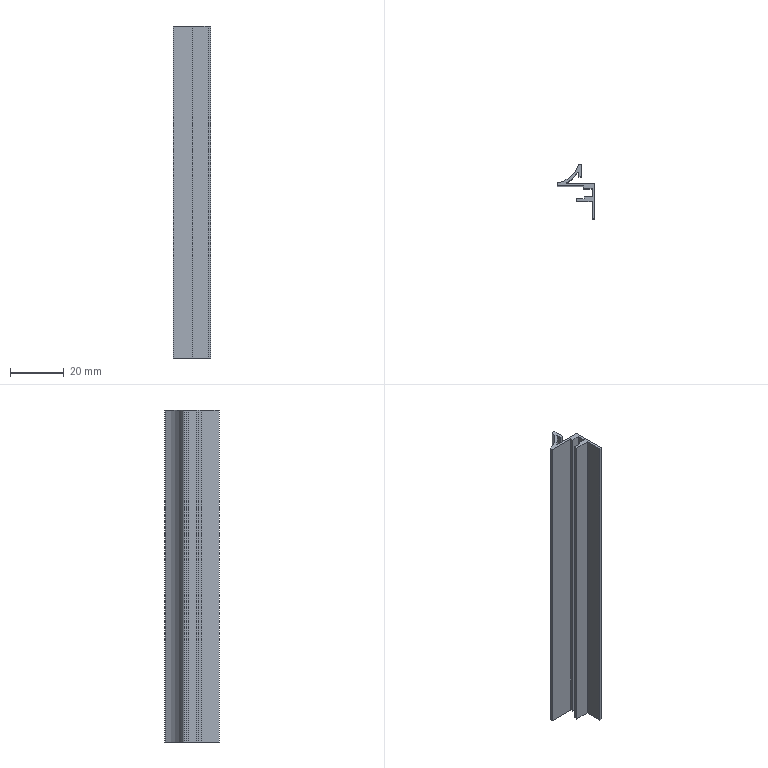Part | SolidWorks | features BaseBody 1, ICE 1, MoveFace 1 | 1 solid | 27 faces | box 14 x 20.3 x 124 mm | volume 6314 mm3 | plane 20 | cylinder 7 | commonest cylinder face diameters 0.387 x2 0.8 x2 0.4 x1 20 x1 22 x1
STEP:
#1=CARTESIAN_POINT('',(-5.304,-0.625,200.));
#2=VERTEX_POINT('',#1);
#3=CARTESIAN_POINT('',(-5.449,-0.8125,200.));
#4=VERTEX_POINT('',#3);
#5=CARTESIAN_POINT('',(-5.255,-0.8125,200.));
#6=DIRECTION('',(0.,0.,1.));
#7=DIRECTION('',(-1.,0.,0.));
#8=AXIS2_PLACEMENT_3D('',#5,#6,#7);
#9=CIRCLE('',#8,0.1937);
#10=EDGE_CURVE('',#2,#4,#9,.T.);
#11=ORIENTED_EDGE('',*,*,#10,.T.);
#12=CARTESIAN_POINT('',(-5.449,-0.8125,76.));
#13=VERTEX_POINT('',#12);
#14=CARTESIAN_POINT('',(-5.449,-0.8125,230.));
#15=DIRECTION('',(0.,0.,-1.));
#16=VECTOR('',#15,1000.);
#17=LINE('',#14,#16);
#18=EDGE_CURVE('',#4,#13,#17,.T.);
#19=ORIENTED_EDGE('',*,*,#18,.T.);
#20=CARTESIAN_POINT('',(-5.304,-0.625,76.));
#21=VERTEX_POINT('',#20);
#22=CARTESIAN_POINT('',(-5.255,-0.8125,76.));
#23=DIRECTION('',(0.,0.,-1.));
#24=DIRECTION('',(1.,0.,0.));
#25=AXIS2_PLACEMENT_3D('',#22,#23,#24);
#26=CIRCLE('',#25,0.1937);
#27=EDGE_CURVE('',#13,#21,#26,.T.);
#28=ORIENTED_EDGE('',*,*,#27,.T.);
#29=CARTESIAN_POINT('',(-5.304,-0.625,230.));
#30=DIRECTION('',(0.,0.,-1.));
#31=VECTOR('',#30,1000.);
#32=LINE('',#29,#31);
#33=EDGE_CURVE('',#2,#21,#32,.T.);
#34=ORIENTED_EDGE('',*,*,#33,.F.);
#35=EDGE_LOOP('',(#11,#19,#28,#34));
#36=FACE_OUTER_BOUND('',#35,.T.);
#37=CARTESIAN_POINT('',(-5.255,-0.8125,230.));
#38=DIRECTION('',(0.,0.,-1.));
#39=DIRECTION('',(-1.,0.,0.));
#40=AXIS2_PLACEMENT_3D('',#37,#38,#39);
#41=CYLINDRICAL_SURFACE('',#40,0.1937);
#42=ADVANCED_FACE('',(#36),#41,.F.);
#43=CARTESIAN_POINT('',(5.,-1.,76.));
#44=VERTEX_POINT('',#43);
#45=CARTESIAN_POINT('',(5.,-14.3,76.));
#46=VERTEX_POINT('',#45);
#47=CARTESIAN_POINT('',(5.,29.623,76.));
#48=DIRECTION('',(0.,-1.,0.));
#49=VECTOR('',#48,1000.);
#50=LINE('',#47,#49);
#51=EDGE_CURVE('',#44,#46,#50,.T.);
#52=ORIENTED_EDGE('',*,*,#51,.F.);
#53=CARTESIAN_POINT('',(5.,-1.,200.));
#54=VERTEX_POINT('',#53);
#55=CARTESIAN_POINT('',(5.,-1.,230.));
#56=DIRECTION('',(0.,0.,-1.));
#57=VECTOR('',#56,1000.);
#58=LINE('',#55,#57);
#59=EDGE_CURVE('',#54,#44,#58,.T.);
#60=ORIENTED_EDGE('',*,*,#59,.F.);
#61=CARTESIAN_POINT('',(5.,-14.3,200.));
#62=VERTEX_POINT('',#61);
#63=CARTESIAN_POINT('',(5.,-14.3,200.));
#64=DIRECTION('',(0.,1.,0.));
#65=VECTOR('',#64,1000.);
#66=LINE('',#63,#65);
#67=EDGE_CURVE('',#62,#54,#66,.T.);
#68=ORIENTED_EDGE('',*,*,#67,.F.);
#69=CARTESIAN_POINT('',(5.,-14.3,230.));
#70=DIRECTION('',(0.,0.,1.));
#71=VECTOR('',#70,1000.);
#72=LINE('',#69,#71);
#73=EDGE_CURVE('',#46,#62,#72,.T.);
#74=ORIENTED_EDGE('',*,*,#73,.F.);
#75=EDGE_LOOP('',(#52,#60,#68,#74));
#76=FACE_OUTER_BOUND('',#75,.T.);
#77=CARTESIAN_POINT('',(5.,-14.3,230.));
#78=DIRECTION('',(-1.,0.,0.));
#79=DIRECTION('',(0.,0.,1.));
#80=AXIS2_PLACEMENT_3D('',#77,#78,#79);
#81=PLANE('',#80);
#82=ADVANCED_FACE('',(#76),#81,.F.);
#83=CARTESIAN_POINT('',(-9.,-2.,76.));
#84=VERTEX_POINT('',#83);
#85=CARTESIAN_POINT('',(-9.,-2.,200.));
#86=VERTEX_POINT('',#85);
#87=CARTESIAN_POINT('',(-9.,-2.,230.));
#88=DIRECTION('',(0.,0.,1.));
#89=VECTOR('',#88,1000.);
#90=LINE('',#87,#89);
#91=EDGE_CURVE('',#84,#86,#90,.T.);
#92=ORIENTED_EDGE('',*,*,#91,.F.);
#93=CARTESIAN_POINT('',(0.9,-2.,76.));
#94=VERTEX_POINT('',#93);
#95=CARTESIAN_POINT('',(5.,-2.,76.));
#96=DIRECTION('',(-1.,0.,0.));
#97=VECTOR('',#96,1000.);
#98=LINE('',#95,#97);
#99=EDGE_CURVE('',#94,#84,#98,.T.);
#100=ORIENTED_EDGE('',*,*,#99,.F.);
#101=CARTESIAN_POINT('',(0.9,-2.,200.));
#102=VERTEX_POINT('',#101);
#103=CARTESIAN_POINT('',(0.9,-2.,230.));
#104=DIRECTION('',(0.,0.,-1.));
#105=VECTOR('',#104,1000.);
#106=LINE('',#103,#105);
#107=EDGE_CURVE('',#102,#94,#106,.T.);
#108=ORIENTED_EDGE('',*,*,#107,.F.);
#109=CARTESIAN_POINT('',(5.,-2.,200.));
#110=DIRECTION('',(1.,0.,0.));
#111=VECTOR('',#110,1000.);
#112=LINE('',#109,#111);
#113=EDGE_CURVE('',#86,#102,#112,.T.);
#114=ORIENTED_EDGE('',*,*,#113,.F.);
#115=EDGE_LOOP('',(#92,#100,#108,#114));
#116=FACE_OUTER_BOUND('',#115,.T.);
#117=CARTESIAN_POINT('',(-9.,-2.,230.));
#118=DIRECTION('',(0.,1.,0.));
#119=DIRECTION('',(0.,0.,1.));
#120=AXIS2_PLACEMENT_3D('',#117,#118,#119);
#121=PLANE('',#120);
#122=ADVANCED_FACE('',(#116),#121,.F.);
#123=CARTESIAN_POINT('',(4.,-6.,200.));
#124=VERTEX_POINT('',#123);
#125=CARTESIAN_POINT('',(4.,-3.,200.));
#126=VERTEX_POINT('',#125);
#127=CARTESIAN_POINT('',(4.,29.623,200.));
#128=DIRECTION('',(0.,1.,0.));
#129=VECTOR('',#128,1000.);
#130=LINE('',#127,#129);
#131=EDGE_CURVE('',#124,#126,#130,.T.);
#132=ORIENTED_EDGE('',*,*,#131,.F.);
#133=CARTESIAN_POINT('',(1.,-6.,200.));
#134=VERTEX_POINT('',#133);
#135=CARTESIAN_POINT('',(5.,-6.,200.));
#136=DIRECTION('',(1.,0.,0.));
#137=VECTOR('',#136,1000.);
#138=LINE('',#135,#137);
#139=EDGE_CURVE('',#134,#124,#138,.T.);
#140=ORIENTED_EDGE('',*,*,#139,.F.);
#141=CARTESIAN_POINT('',(1.,-6.7,200.));
#142=VERTEX_POINT('',#141);
#143=CARTESIAN_POINT('',(1.,-6.,200.));
#144=DIRECTION('',(0.,-1.,0.));
#145=VECTOR('',#144,1000.);
#146=LINE('',#143,#145);
#147=EDGE_CURVE('',#134,#142,#146,.T.);
#148=ORIENTED_EDGE('',*,*,#147,.T.);
#149=CARTESIAN_POINT('',(-1.7,-6.7,200.));
#150=VERTEX_POINT('',#149);
#151=CARTESIAN_POINT('',(5.,-6.7,200.));
#152=DIRECTION('',(1.,0.,0.));
#153=VECTOR('',#152,1000.);
#154=LINE('',#151,#153);
#155=EDGE_CURVE('',#150,#142,#154,.T.);
#156=ORIENTED_EDGE('',*,*,#155,.F.);
#157=CARTESIAN_POINT('',(-1.7,-7.7,200.));
#158=VERTEX_POINT('',#157);
#159=CARTESIAN_POINT('',(-1.7,-6.7,200.));
#160=DIRECTION('',(0.,-1.,0.));
#161=VECTOR('',#160,1000.);
#162=LINE('',#159,#161);
#163=EDGE_CURVE('',#150,#158,#162,.T.);
#164=ORIENTED_EDGE('',*,*,#163,.T.);
#165=CARTESIAN_POINT('',(4.,-7.7,200.));
#166=VERTEX_POINT('',#165);
#167=CARTESIAN_POINT('',(5.,-7.7,200.));
#168=DIRECTION('',(-1.,0.,0.));
#169=VECTOR('',#168,1000.);
#170=LINE('',#167,#169);
#171=EDGE_CURVE('',#166,#158,#170,.T.);
#172=ORIENTED_EDGE('',*,*,#171,.F.);
#173=CARTESIAN_POINT('',(4.,-14.3,200.));
#174=VERTEX_POINT('',#173);
#175=CARTESIAN_POINT('',(4.,29.623,200.));
#176=DIRECTION('',(0.,1.,0.));
#177=VECTOR('',#176,1000.);
#178=LINE('',#175,#177);
#179=EDGE_CURVE('',#174,#166,#178,.T.);
#180=ORIENTED_EDGE('',*,*,#179,.F.);
#181=CARTESIAN_POINT('',(5.,-14.3,200.));
#182=DIRECTION('',(-1.,0.,0.));
#183=VECTOR('',#182,1000.);
#184=LINE('',#181,#183);
#185=EDGE_CURVE('',#62,#174,#184,.T.);
#186=ORIENTED_EDGE('',*,*,#185,.F.);
#187=ORIENTED_EDGE('',*,*,#67,.T.);
#188=CARTESIAN_POINT('',(-5.207,-1.,200.));
#189=VERTEX_POINT('',#188);
#190=CARTESIAN_POINT('',(5.,-1.,200.));
#191=DIRECTION('',(1.,0.,0.));
#192=VECTOR('',#191,1000.);
#193=LINE('',#190,#192);
#194=EDGE_CURVE('',#189,#54,#193,.T.);
#195=ORIENTED_EDGE('',*,*,#194,.F.);
#196=CARTESIAN_POINT('',(-5.255,-0.8125,200.));
#197=DIRECTION('',(0.,0.,1.));
#198=DIRECTION('',(-1.,0.,0.));
#199=AXIS2_PLACEMENT_3D('',#196,#197,#198);
#200=CIRCLE('',#199,0.1937);
#201=EDGE_CURVE('',#4,#189,#200,.T.);
#202=ORIENTED_EDGE('',*,*,#201,.F.);
#203=ORIENTED_EDGE('',*,*,#10,.F.);
#204=CARTESIAN_POINT('',(-1.368,3.063,200.));
#205=VERTEX_POINT('',#204);
#206=CARTESIAN_POINT('',(-10.628,9.,200.));
#207=DIRECTION('',(0.,0.,1.));
#208=DIRECTION('',(-1.,0.,0.));
#209=AXIS2_PLACEMENT_3D('',#206,#207,#208);
#210=CIRCLE('',#209,11.);
#211=EDGE_CURVE('',#2,#205,#210,.T.);
#212=ORIENTED_EDGE('',*,*,#211,.T.);
#213=CARTESIAN_POINT('',(-1.,2.955,200.));
#214=VERTEX_POINT('',#213);
#215=CARTESIAN_POINT('',(-1.2,2.955,200.));
#216=DIRECTION('',(0.,0.,1.));
#217=DIRECTION('',(-1.,0.,0.));
#218=AXIS2_PLACEMENT_3D('',#215,#216,#217);
#219=CIRCLE('',#218,0.2);
#220=EDGE_CURVE('',#214,#205,#219,.T.);
#221=ORIENTED_EDGE('',*,*,#220,.F.);
#222=CARTESIAN_POINT('',(-1.,1.5,200.));
#223=VERTEX_POINT('',#222);
#224=CARTESIAN_POINT('',(-1.,2.955,200.));
#225=DIRECTION('',(0.,1.,0.));
#226=VECTOR('',#225,1000.);
#227=LINE('',#224,#226);
#228=EDGE_CURVE('',#223,#214,#227,.T.);
#229=ORIENTED_EDGE('',*,*,#228,.F.);
#230=CARTESIAN_POINT('',(0.,1.5,200.));
#231=VERTEX_POINT('',#230);
#232=CARTESIAN_POINT('',(-1.,1.5,200.));
#233=DIRECTION('',(-1.,0.,0.));
#234=VECTOR('',#233,1000.);
#235=LINE('',#232,#234);
#236=EDGE_CURVE('',#231,#223,#235,.T.);
#237=ORIENTED_EDGE('',*,*,#236,.F.);
#238=CARTESIAN_POINT('',(0.,6.,200.));
#239=VERTEX_POINT('',#238);
#240=CARTESIAN_POINT('',(0.,1.5,200.));
#241=DIRECTION('',(0.,-1.,0.));
#242=VECTOR('',#241,1000.);
#243=LINE('',#240,#242);
#244=EDGE_CURVE('',#239,#231,#243,.T.);
#245=ORIENTED_EDGE('',*,*,#244,.F.);
#246=CARTESIAN_POINT('',(-0.8,6.,200.));
#247=VERTEX_POINT('',#246);
#248=CARTESIAN_POINT('',(0.,6.,200.));
#249=DIRECTION('',(1.,0.,0.));
#250=VECTOR('',#249,1000.);
#251=LINE('',#248,#250);
#252=EDGE_CURVE('',#247,#239,#251,.T.);
#253=ORIENTED_EDGE('',*,*,#252,.F.);
#254=CARTESIAN_POINT('',(-1.178,5.731,200.));
#255=VERTEX_POINT('',#254);
#256=CARTESIAN_POINT('',(-0.8,5.6,200.));
#257=DIRECTION('',(0.,0.,1.));
#258=DIRECTION('',(-1.,0.,0.));
#259=AXIS2_PLACEMENT_3D('',#256,#257,#258);
#260=CIRCLE('',#259,0.4);
#261=EDGE_CURVE('',#247,#255,#260,.T.);
#262=ORIENTED_EDGE('',*,*,#261,.T.);
#263=CARTESIAN_POINT('',(-8.678,-0.8077,200.));
#264=VERTEX_POINT('',#263);
#265=CARTESIAN_POINT('',(-10.628,9.,200.));
#266=DIRECTION('',(0.,0.,1.));
#267=DIRECTION('',(-1.,0.,0.));
#268=AXIS2_PLACEMENT_3D('',#265,#266,#267);
#269=CIRCLE('',#268,10.);
#270=EDGE_CURVE('',#264,#255,#269,.T.);
#271=ORIENTED_EDGE('',*,*,#270,.F.);
#272=CARTESIAN_POINT('',(-9.,-1.2,200.));
#273=VERTEX_POINT('',#272);
#274=CARTESIAN_POINT('',(-8.6,-1.2,200.));
#275=DIRECTION('',(0.,0.,1.));
#276=DIRECTION('',(-1.,0.,0.));
#277=AXIS2_PLACEMENT_3D('',#274,#275,#276);
#278=CIRCLE('',#277,0.4);
#279=EDGE_CURVE('',#264,#273,#278,.T.);
#280=ORIENTED_EDGE('',*,*,#279,.T.);
#281=CARTESIAN_POINT('',(-9.,8.,200.));
#282=DIRECTION('',(0.,-1.,0.));
#283=VECTOR('',#282,1000.);
#284=LINE('',#281,#283);
#285=EDGE_CURVE('',#273,#86,#284,.T.);
#286=ORIENTED_EDGE('',*,*,#285,.T.);
#287=ORIENTED_EDGE('',*,*,#113,.T.);
#288=CARTESIAN_POINT('',(0.9,-3.,200.));
#289=VERTEX_POINT('',#288);
#290=CARTESIAN_POINT('',(0.9,29.623,200.));
#291=DIRECTION('',(0.,1.,0.));
#292=VECTOR('',#291,1000.);
#293=LINE('',#290,#292);
#294=EDGE_CURVE('',#289,#102,#293,.T.);
#295=ORIENTED_EDGE('',*,*,#294,.F.);
#296=CARTESIAN_POINT('',(5.,-3.,200.));
#297=DIRECTION('',(-1.,0.,0.));
#298=VECTOR('',#297,1000.);
#299=LINE('',#296,#298);
#300=EDGE_CURVE('',#126,#289,#299,.T.);
#301=ORIENTED_EDGE('',*,*,#300,.F.);
#302=EDGE_LOOP('',(#132,#140,#148,#156,#164,#172,#180,#186,#187,#195,#202,#203,#212,#221,#229,#237,#245,#253,#262,#271,#280,#286,#287,#295,#301));
#303=FACE_OUTER_BOUND('',#302,.T.);
#304=CARTESIAN_POINT('',(5.,29.623,200.));
#305=DIRECTION('',(0.,0.,-1.));
#306=DIRECTION('',(-1.,0.,0.));
#307=AXIS2_PLACEMENT_3D('',#304,#305,#306);
#308=PLANE('',#307);
#309=ADVANCED_FACE('',(#303),#308,.F.);
#310=ORIENTED_EDGE('',*,*,#185,.T.);
#311=CARTESIAN_POINT('',(4.,-14.3,76.));
#312=VERTEX_POINT('',#311);
#313=CARTESIAN_POINT('',(4.,-14.3,230.));
#314=DIRECTION('',(0.,0.,1.));
#315=VECTOR('',#314,1000.);
#316=LINE('',#313,#315);
#317=EDGE_CURVE('',#312,#174,#316,.T.);
#318=ORIENTED_EDGE('',*,*,#317,.F.);
#319=CARTESIAN_POINT('',(5.,-14.3,76.));
#320=DIRECTION('',(-1.,0.,0.));
#321=VECTOR('',#320,1000.);
#322=LINE('',#319,#321);
#323=EDGE_CURVE('',#46,#312,#322,.T.);
#324=ORIENTED_EDGE('',*,*,#323,.F.);
#325=ORIENTED_EDGE('',*,*,#73,.T.);
#326=EDGE_LOOP('',(#310,#318,#324,#325));
#327=FACE_OUTER_BOUND('',#326,.T.);
#328=CARTESIAN_POINT('',(4.,-14.3,230.));
#329=DIRECTION('',(0.,1.,0.));
#330=DIRECTION('',(0.,0.,1.));
#331=AXIS2_PLACEMENT_3D('',#328,#329,#330);
#332=PLANE('',#331);
#333=ADVANCED_FACE('',(#327),#332,.F.);
#334=ORIENTED_EDGE('',*,*,#51,.T.);
#335=ORIENTED_EDGE('',*,*,#323,.T.);
#336=CARTESIAN_POINT('',(4.,-7.7,76.));
#337=VERTEX_POINT('',#336);
#338=CARTESIAN_POINT('',(4.,-7.7,76.));
#339=DIRECTION('',(0.,-1.,0.));
#340=VECTOR('',#339,1000.);
#341=LINE('',#338,#340);
#342=EDGE_CURVE('',#337,#312,#341,.T.);
#343=ORIENTED_EDGE('',*,*,#342,.F.);
#344=CARTESIAN_POINT('',(-1.7,-7.7,76.));
#345=VERTEX_POINT('',#344);
#346=CARTESIAN_POINT('',(-1.7,-7.7,76.));
#347=DIRECTION('',(1.,0.,0.));
#348=VECTOR('',#347,1000.);
#349=LINE('',#346,#348);
#350=EDGE_CURVE('',#345,#337,#349,.T.);
#351=ORIENTED_EDGE('',*,*,#350,.F.);
#352=CARTESIAN_POINT('',(-1.7,-6.7,76.));
#353=VERTEX_POINT('',#352);
#354=CARTESIAN_POINT('',(-1.7,29.623,76.));
#355=DIRECTION('',(0.,1.,0.));
#356=VECTOR('',#355,1000.);
#357=LINE('',#354,#356);
#358=EDGE_CURVE('',#345,#353,#357,.T.);
#359=ORIENTED_EDGE('',*,*,#358,.T.);
#360=CARTESIAN_POINT('',(1.,-6.7,76.));
#361=VERTEX_POINT('',#360);
#362=CARTESIAN_POINT('',(1.,-6.7,76.));
#363=DIRECTION('',(-1.,0.,0.));
#364=VECTOR('',#363,1000.);
#365=LINE('',#362,#364);
#366=EDGE_CURVE('',#361,#353,#365,.T.);
#367=ORIENTED_EDGE('',*,*,#366,.F.);
#368=CARTESIAN_POINT('',(1.,-6.,76.));
#369=VERTEX_POINT('',#368);
#370=CARTESIAN_POINT('',(1.,29.623,76.));
#371=DIRECTION('',(0.,1.,0.));
#372=VECTOR('',#371,1000.);
#373=LINE('',#370,#372);
#374=EDGE_CURVE('',#361,#369,#373,.T.);
#375=ORIENTED_EDGE('',*,*,#374,.T.);
#376=CARTESIAN_POINT('',(4.,-6.,76.));
#377=VERTEX_POINT('',#376);
#378=CARTESIAN_POINT('',(4.,-6.,76.));
#379=DIRECTION('',(-1.,0.,0.));
#380=VECTOR('',#379,1000.);
#381=LINE('',#378,#380);
#382=EDGE_CURVE('',#377,#369,#381,.T.);
#383=ORIENTED_EDGE('',*,*,#382,.F.);
#384=CARTESIAN_POINT('',(4.,-3.,76.));
#385=VERTEX_POINT('',#384);
#386=CARTESIAN_POINT('',(4.,-3.,76.));
#387=DIRECTION('',(0.,-1.,0.));
#388=VECTOR('',#387,1000.);
#389=LINE('',#386,#388);
#390=EDGE_CURVE('',#385,#377,#389,.T.);
#391=ORIENTED_EDGE('',*,*,#390,.F.);
#392=CARTESIAN_POINT('',(0.9,-3.,76.));
#393=VERTEX_POINT('',#392);
#394=CARTESIAN_POINT('',(0.9,-3.,76.));
#395=DIRECTION('',(1.,0.,0.));
#396=VECTOR('',#395,1000.);
#397=LINE('',#394,#396);
#398=EDGE_CURVE('',#393,#385,#397,.T.);
#399=ORIENTED_EDGE('',*,*,#398,.F.);
#400=CARTESIAN_POINT('',(0.9,-2.,76.));
#401=DIRECTION('',(0.,-1.,0.));
#402=VECTOR('',#401,1000.);
#403=LINE('',#400,#402);
#404=EDGE_CURVE('',#94,#393,#403,.T.);
#405=ORIENTED_EDGE('',*,*,#404,.F.);
#406=ORIENTED_EDGE('',*,*,#99,.T.);
#407=CARTESIAN_POINT('',(-9.,-1.2,76.));
#408=VERTEX_POINT('',#407);
#409=CARTESIAN_POINT('',(-9.,-1.2,76.));
#410=DIRECTION('',(0.,-1.,0.));
#411=VECTOR('',#410,1000.);
#412=LINE('',#409,#411);
#413=EDGE_CURVE('',#408,#84,#412,.T.);
#414=ORIENTED_EDGE('',*,*,#413,.F.);
#415=CARTESIAN_POINT('',(-8.678,-0.8077,76.));
#416=VERTEX_POINT('',#415);
#417=CARTESIAN_POINT('',(-8.6,-1.2,76.));
#418=DIRECTION('',(0.,0.,-1.));
#419=DIRECTION('',(1.,0.,0.));
#420=AXIS2_PLACEMENT_3D('',#417,#418,#419);
#421=CIRCLE('',#420,0.4);
#422=EDGE_CURVE('',#408,#416,#421,.T.);
#423=ORIENTED_EDGE('',*,*,#422,.T.);
#424=CARTESIAN_POINT('',(-1.178,5.731,76.));
#425=VERTEX_POINT('',#424);
#426=CARTESIAN_POINT('',(-10.628,9.,76.));
#427=DIRECTION('',(0.,0.,-1.));
#428=DIRECTION('',(1.,0.,0.));
#429=AXIS2_PLACEMENT_3D('',#426,#427,#428);
#430=CIRCLE('',#429,10.);
#431=EDGE_CURVE('',#425,#416,#430,.T.);
#432=ORIENTED_EDGE('',*,*,#431,.F.);
#433=CARTESIAN_POINT('',(-0.8,6.,76.));
#434=VERTEX_POINT('',#433);
#435=CARTESIAN_POINT('',(-0.8,5.6,76.));
#436=DIRECTION('',(0.,0.,-1.));
#437=DIRECTION('',(1.,0.,0.));
#438=AXIS2_PLACEMENT_3D('',#435,#436,#437);
#439=CIRCLE('',#438,0.4);
#440=EDGE_CURVE('',#425,#434,#439,.T.);
#441=ORIENTED_EDGE('',*,*,#440,.T.);
#442=CARTESIAN_POINT('',(0.,6.,76.));
#443=VERTEX_POINT('',#442);
#444=CARTESIAN_POINT('',(0.,6.,76.));
#445=DIRECTION('',(-1.,0.,0.));
#446=VECTOR('',#445,1000.);
#447=LINE('',#444,#446);
#448=EDGE_CURVE('',#443,#434,#447,.T.);
#449=ORIENTED_EDGE('',*,*,#448,.F.);
#450=CARTESIAN_POINT('',(0.,1.5,76.));
#451=VERTEX_POINT('',#450);
#452=CARTESIAN_POINT('',(0.,1.5,76.));
#453=DIRECTION('',(0.,1.,0.));
#454=VECTOR('',#453,1000.);
#455=LINE('',#452,#454);
#456=EDGE_CURVE('',#451,#443,#455,.T.);
#457=ORIENTED_EDGE('',*,*,#456,.F.);
#458=CARTESIAN_POINT('',(-1.,1.5,76.));
#459=VERTEX_POINT('',#458);
#460=CARTESIAN_POINT('',(-1.,1.5,76.));
#461=DIRECTION('',(1.,0.,0.));
#462=VECTOR('',#461,1000.);
#463=LINE('',#460,#462);
#464=EDGE_CURVE('',#459,#451,#463,.T.);
#465=ORIENTED_EDGE('',*,*,#464,.F.);
#466=CARTESIAN_POINT('',(-1.,2.955,76.));
#467=VERTEX_POINT('',#466);
#468=CARTESIAN_POINT('',(-1.,2.955,76.));
#469=DIRECTION('',(0.,-1.,0.));
#470=VECTOR('',#469,1000.);
#471=LINE('',#468,#470);
#472=EDGE_CURVE('',#467,#459,#471,.T.);
#473=ORIENTED_EDGE('',*,*,#472,.F.);
#474=CARTESIAN_POINT('',(-1.368,3.063,76.));
#475=VERTEX_POINT('',#474);
#476=CARTESIAN_POINT('',(-1.2,2.955,76.));
#477=DIRECTION('',(0.,0.,-1.));
#478=DIRECTION('',(1.,0.,0.));
#479=AXIS2_PLACEMENT_3D('',#476,#477,#478);
#480=CIRCLE('',#479,0.2);
#481=EDGE_CURVE('',#475,#467,#480,.T.);
#482=ORIENTED_EDGE('',*,*,#481,.F.);
#483=CARTESIAN_POINT('',(-10.628,9.,76.));
#484=DIRECTION('',(0.,0.,-1.));
#485=DIRECTION('',(1.,0.,0.));
#486=AXIS2_PLACEMENT_3D('',#483,#484,#485);
#487=CIRCLE('',#486,11.);
#488=EDGE_CURVE('',#475,#21,#487,.T.);
#489=ORIENTED_EDGE('',*,*,#488,.T.);
#490=ORIENTED_EDGE('',*,*,#27,.F.);
#491=CARTESIAN_POINT('',(-5.207,-1.,76.));
#492=VERTEX_POINT('',#491);
#493=CARTESIAN_POINT('',(-5.255,-0.8125,76.));
#494=DIRECTION('',(0.,0.,-1.));
#495=DIRECTION('',(1.,0.,0.));
#496=AXIS2_PLACEMENT_3D('',#493,#494,#495);
#497=CIRCLE('',#496,0.1937);
#498=EDGE_CURVE('',#492,#13,#497,.T.);
#499=ORIENTED_EDGE('',*,*,#498,.F.);
#500=CARTESIAN_POINT('',(5.,-1.,76.));
#501=DIRECTION('',(-1.,0.,0.));
#502=VECTOR('',#501,1000.);
#503=LINE('',#500,#502);
#504=EDGE_CURVE('',#44,#492,#503,.T.);
#505=ORIENTED_EDGE('',*,*,#504,.F.);
#506=EDGE_LOOP('',(#334,#335,#343,#351,#359,#367,#375,#383,#391,#399,#405,#406,#414,#423,#432,#441,#449,#457,#465,#473,#482,#489,#490,#499,#505));
#507=FACE_OUTER_BOUND('',#506,.T.);
#508=CARTESIAN_POINT('',(5.,29.623,76.));
#509=DIRECTION('',(0.,0.,1.));
#510=DIRECTION('',(1.,0.,0.));
#511=AXIS2_PLACEMENT_3D('',#508,#509,#510);
#512=PLANE('',#511);
#513=ADVANCED_FACE('',(#507),#512,.F.);
#514=ORIENTED_EDGE('',*,*,#59,.T.);
#515=ORIENTED_EDGE('',*,*,#504,.T.);
#516=CARTESIAN_POINT('',(-5.207,-1.,230.));
#517=DIRECTION('',(0.,0.,-1.));
#518=VECTOR('',#517,1000.);
#519=LINE('',#516,#518);
#520=EDGE_CURVE('',#189,#492,#519,.T.);
#521=ORIENTED_EDGE('',*,*,#520,.F.);
#522=ORIENTED_EDGE('',*,*,#194,.T.);
#523=EDGE_LOOP('',(#514,#515,#521,#522));
#524=FACE_OUTER_BOUND('',#523,.T.);
#525=CARTESIAN_POINT('',(5.,-1.,230.));
#526=DIRECTION('',(0.,-1.,0.));
#527=DIRECTION('',(0.,0.,-1.));
#528=AXIS2_PLACEMENT_3D('',#525,#526,#527);
#529=PLANE('',#528);
#530=ADVANCED_FACE('',(#524),#529,.F.);
#531=CARTESIAN_POINT('',(-9.,-1.2,230.));
#532=DIRECTION('',(0.,0.,1.));
#533=VECTOR('',#532,1000.);
#534=LINE('',#531,#533);
#535=EDGE_CURVE('',#408,#273,#534,.T.);
#536=ORIENTED_EDGE('',*,*,#535,.F.);
#537=ORIENTED_EDGE('',*,*,#413,.T.);
#538=ORIENTED_EDGE('',*,*,#91,.T.);
#539=ORIENTED_EDGE('',*,*,#285,.F.);
#540=EDGE_LOOP('',(#536,#537,#538,#539));
#541=FACE_OUTER_BOUND('',#540,.T.);
#542=CARTESIAN_POINT('',(-9.,-1.2,230.));
#543=DIRECTION('',(1.,0.,0.));
#544=DIRECTION('',(0.,0.,-1.));
#545=AXIS2_PLACEMENT_3D('',#542,#543,#544);
#546=PLANE('',#545);
#547=ADVANCED_FACE('',(#541),#546,.F.);
#548=ORIENTED_EDGE('',*,*,#294,.T.);
#549=ORIENTED_EDGE('',*,*,#107,.T.);
#550=ORIENTED_EDGE('',*,*,#404,.T.);
#551=CARTESIAN_POINT('',(0.9,-3.,230.));
#552=DIRECTION('',(0.,0.,-1.));
#553=VECTOR('',#552,1000.);
#554=LINE('',#551,#553);
#555=EDGE_CURVE('',#289,#393,#554,.T.);
#556=ORIENTED_EDGE('',*,*,#555,.F.);
#557=EDGE_LOOP('',(#548,#549,#550,#556));
#558=FACE_OUTER_BOUND('',#557,.T.);
#559=CARTESIAN_POINT('',(0.9,-2.,230.));
#560=DIRECTION('',(1.,0.,0.));
#561=DIRECTION('',(0.,0.,-1.));
#562=AXIS2_PLACEMENT_3D('',#559,#560,#561);
#563=PLANE('',#562);
#564=ADVANCED_FACE('',(#558),#563,.F.);
#565=ORIENTED_EDGE('',*,*,#300,.T.);
#566=ORIENTED_EDGE('',*,*,#555,.T.);
#567=ORIENTED_EDGE('',*,*,#398,.T.);
#568=CARTESIAN_POINT('',(4.,-3.,230.));
#569=DIRECTION('',(0.,0.,-1.));
#570=VECTOR('',#569,1000.);
#571=LINE('',#568,#570);
#572=EDGE_CURVE('',#126,#385,#571,.T.);
#573=ORIENTED_EDGE('',*,*,#572,.F.);
#574=EDGE_LOOP('',(#565,#566,#567,#573));
#575=FACE_OUTER_BOUND('',#574,.T.);
#576=CARTESIAN_POINT('',(0.9,-3.,230.));
#577=DIRECTION('',(0.,1.,0.));
#578=DIRECTION('',(0.,0.,1.));
#579=AXIS2_PLACEMENT_3D('',#576,#577,#578);
#580=PLANE('',#579);
#581=ADVANCED_FACE('',(#575),#580,.F.);
#582=ORIENTED_EDGE('',*,*,#131,.T.);
#583=ORIENTED_EDGE('',*,*,#572,.T.);
#584=ORIENTED_EDGE('',*,*,#390,.T.);
#585=CARTESIAN_POINT('',(4.,-6.,230.));
#586=DIRECTION('',(0.,0.,-1.));
#587=VECTOR('',#586,1000.);
#588=LINE('',#585,#587);
#589=EDGE_CURVE('',#124,#377,#588,.T.);
#590=ORIENTED_EDGE('',*,*,#589,.F.);
#591=EDGE_LOOP('',(#582,#583,#584,#590));
#592=FACE_OUTER_BOUND('',#591,.T.);
#593=CARTESIAN_POINT('',(4.,-3.,230.));
#594=DIRECTION('',(1.,0.,0.));
#595=DIRECTION('',(0.,0.,-1.));
#596=AXIS2_PLACEMENT_3D('',#593,#594,#595);
#597=PLANE('',#596);
#598=ADVANCED_FACE('',(#592),#597,.F.);
#599=ORIENTED_EDGE('',*,*,#139,.T.);
#600=ORIENTED_EDGE('',*,*,#589,.T.);
#601=ORIENTED_EDGE('',*,*,#382,.T.);
#602=CARTESIAN_POINT('',(1.,-6.,230.));
#603=DIRECTION('',(0.,0.,-1.));
#604=VECTOR('',#603,1000.);
#605=LINE('',#602,#604);
#606=EDGE_CURVE('',#134,#369,#605,.T.);
#607=ORIENTED_EDGE('',*,*,#606,.F.);
#608=EDGE_LOOP('',(#599,#600,#601,#607));
#609=FACE_OUTER_BOUND('',#608,.T.);
#610=CARTESIAN_POINT('',(4.,-6.,230.));
#611=DIRECTION('',(0.,-1.,0.));
#612=DIRECTION('',(0.,0.,-1.));
#613=AXIS2_PLACEMENT_3D('',#610,#611,#612);
#614=PLANE('',#613);
#615=ADVANCED_FACE('',(#609),#614,.F.);
#616=ORIENTED_EDGE('',*,*,#155,.T.);
#617=CARTESIAN_POINT('',(1.,-6.7,230.));
#618=DIRECTION('',(0.,0.,1.));
#619=VECTOR('',#618,1000.);
#620=LINE('',#617,#619);
#621=EDGE_CURVE('',#361,#142,#620,.T.);
#622=ORIENTED_EDGE('',*,*,#621,.F.);
#623=ORIENTED_EDGE('',*,*,#366,.T.);
#624=CARTESIAN_POINT('',(-1.7,-6.7,230.));
#625=DIRECTION('',(0.,0.,-1.));
#626=VECTOR('',#625,1000.);
#627=LINE('',#624,#626);
#628=EDGE_CURVE('',#150,#353,#627,.T.);
#629=ORIENTED_EDGE('',*,*,#628,.F.);
#630=EDGE_LOOP('',(#616,#622,#623,#629));
#631=FACE_OUTER_BOUND('',#630,.T.);
#632=CARTESIAN_POINT('',(1.,-6.7,230.));
#633=DIRECTION('',(0.,-1.,0.));
#634=DIRECTION('',(0.,0.,-1.));
#635=AXIS2_PLACEMENT_3D('',#632,#633,#634);
#636=PLANE('',#635);
#637=ADVANCED_FACE('',(#631),#636,.F.);
#638=ORIENTED_EDGE('',*,*,#171,.T.);
#639=CARTESIAN_POINT('',(-1.7,-7.7,230.));
#640=DIRECTION('',(0.,0.,1.));
#641=VECTOR('',#640,1000.);
#642=LINE('',#639,#641);
#643=EDGE_CURVE('',#345,#158,#642,.T.);
#644=ORIENTED_EDGE('',*,*,#643,.F.);
#645=ORIENTED_EDGE('',*,*,#350,.T.);
#646=CARTESIAN_POINT('',(4.,-7.7,230.));
#647=DIRECTION('',(0.,0.,-1.));
#648=VECTOR('',#647,1000.);
#649=LINE('',#646,#648);
#650=EDGE_CURVE('',#166,#337,#649,.T.);
#651=ORIENTED_EDGE('',*,*,#650,.F.);
#652=EDGE_LOOP('',(#638,#644,#645,#651));
#653=FACE_OUTER_BOUND('',#652,.T.);
#654=CARTESIAN_POINT('',(-1.7,-7.7,230.));
#655=DIRECTION('',(0.,1.,0.));
#656=DIRECTION('',(0.,0.,1.));
#657=AXIS2_PLACEMENT_3D('',#654,#655,#656);
#658=PLANE('',#657);
#659=ADVANCED_FACE('',(#653),#658,.F.);
#660=ORIENTED_EDGE('',*,*,#179,.T.);
#661=ORIENTED_EDGE('',*,*,#650,.T.);
#662=ORIENTED_EDGE('',*,*,#342,.T.);
#663=ORIENTED_EDGE('',*,*,#317,.T.);
#664=EDGE_LOOP('',(#660,#661,#662,#663));
#665=FACE_OUTER_BOUND('',#664,.T.);
#666=CARTESIAN_POINT('',(4.,-7.7,230.));
#667=DIRECTION('',(1.,0.,0.));
#668=DIRECTION('',(0.,0.,-1.));
#669=AXIS2_PLACEMENT_3D('',#666,#667,#668);
#670=PLANE('',#669);
#671=ADVANCED_FACE('',(#665),#670,.F.);
#672=ORIENTED_EDGE('',*,*,#18,.F.);
#673=ORIENTED_EDGE('',*,*,#201,.T.);
#674=ORIENTED_EDGE('',*,*,#520,.T.);
#675=ORIENTED_EDGE('',*,*,#498,.T.);
#676=EDGE_LOOP('',(#672,#673,#674,#675));
#677=FACE_OUTER_BOUND('',#676,.T.);
#678=CARTESIAN_POINT('',(-5.255,-0.8125,230.));
#679=DIRECTION('',(0.,0.,-1.));
#680=DIRECTION('',(-1.,0.,0.));
#681=AXIS2_PLACEMENT_3D('',#678,#679,#680);
#682=CYLINDRICAL_SURFACE('',#681,0.1937);
#683=ADVANCED_FACE('',(#677),#682,.F.);
#684=CARTESIAN_POINT('',(-1.,2.955,230.));
#685=DIRECTION('',(0.,0.,1.));
#686=VECTOR('',#685,1000.);
#687=LINE('',#684,#686);
#688=EDGE_CURVE('',#467,#214,#687,.T.);
#689=ORIENTED_EDGE('',*,*,#688,.F.);
#690=ORIENTED_EDGE('',*,*,#472,.T.);
#691=CARTESIAN_POINT('',(-1.,1.5,230.));
#692=DIRECTION('',(0.,0.,-1.));
#693=VECTOR('',#692,1000.);
#694=LINE('',#691,#693);
#695=EDGE_CURVE('',#223,#459,#694,.T.);
#696=ORIENTED_EDGE('',*,*,#695,.F.);
#697=ORIENTED_EDGE('',*,*,#228,.T.);
#698=EDGE_LOOP('',(#689,#690,#696,#697));
#699=FACE_OUTER_BOUND('',#698,.T.);
#700=CARTESIAN_POINT('',(-1.,2.955,230.));
#701=DIRECTION('',(1.,0.,0.));
#702=DIRECTION('',(0.,0.,-1.));
#703=AXIS2_PLACEMENT_3D('',#700,#701,#702);
#704=PLANE('',#703);
#705=ADVANCED_FACE('',(#699),#704,.F.);
#706=ORIENTED_EDGE('',*,*,#488,.F.);
#707=CARTESIAN_POINT('',(-1.368,3.063,230.));
#708=DIRECTION('',(0.,0.,1.));
#709=VECTOR('',#708,1000.);
#710=LINE('',#707,#709);
#711=EDGE_CURVE('',#475,#205,#710,.T.);
#712=ORIENTED_EDGE('',*,*,#711,.T.);
#713=ORIENTED_EDGE('',*,*,#211,.F.);
#714=ORIENTED_EDGE('',*,*,#33,.T.);
#715=EDGE_LOOP('',(#706,#712,#713,#714));
#716=FACE_OUTER_BOUND('',#715,.T.);
#717=CARTESIAN_POINT('',(-10.628,9.,230.));
#718=DIRECTION('',(0.,0.,-1.));
#719=DIRECTION('',(-1.,0.,0.));
#720=AXIS2_PLACEMENT_3D('',#717,#718,#719);
#721=CYLINDRICAL_SURFACE('',#720,11.);
#722=ADVANCED_FACE('',(#716),#721,.T.);
#723=CARTESIAN_POINT('',(-1.178,5.731,230.));
#724=DIRECTION('',(0.,0.,1.));
#725=VECTOR('',#724,1000.);
#726=LINE('',#723,#725);
#727=EDGE_CURVE('',#425,#255,#726,.T.);
#728=ORIENTED_EDGE('',*,*,#727,.F.);
#729=ORIENTED_EDGE('',*,*,#431,.T.);
#730=CARTESIAN_POINT('',(-8.678,-0.8077,230.));
#731=DIRECTION('',(0.,0.,-1.));
#732=VECTOR('',#731,1000.);
#733=LINE('',#730,#732);
#734=EDGE_CURVE('',#264,#416,#733,.T.);
#735=ORIENTED_EDGE('',*,*,#734,.F.);
#736=ORIENTED_EDGE('',*,*,#270,.T.);
#737=EDGE_LOOP('',(#728,#729,#735,#736));
#738=FACE_OUTER_BOUND('',#737,.T.);
#739=CARTESIAN_POINT('',(-10.628,9.,230.));
#740=DIRECTION('',(0.,0.,-1.));
#741=DIRECTION('',(-1.,0.,0.));
#742=AXIS2_PLACEMENT_3D('',#739,#740,#741);
#743=CYLINDRICAL_SURFACE('',#742,10.);
#744=ADVANCED_FACE('',(#738),#743,.F.);
#745=CARTESIAN_POINT('',(0.,1.5,230.));
#746=DIRECTION('',(0.,0.,1.));
#747=VECTOR('',#746,1000.);
#748=LINE('',#745,#747);
#749=EDGE_CURVE('',#451,#231,#748,.T.);
#750=ORIENTED_EDGE('',*,*,#749,.F.);
#751=ORIENTED_EDGE('',*,*,#456,.T.);
#752=CARTESIAN_POINT('',(0.,6.,230.));
#753=DIRECTION('',(0.,0.,-1.));
#754=VECTOR('',#753,1000.);
#755=LINE('',#752,#754);
#756=EDGE_CURVE('',#239,#443,#755,.T.);
#757=ORIENTED_EDGE('',*,*,#756,.F.);
#758=ORIENTED_EDGE('',*,*,#244,.T.);
#759=EDGE_LOOP('',(#750,#751,#757,#758));
#760=FACE_OUTER_BOUND('',#759,.T.);
#761=CARTESIAN_POINT('',(0.,1.5,230.));
#762=DIRECTION('',(-1.,0.,0.));
#763=DIRECTION('',(0.,0.,1.));
#764=AXIS2_PLACEMENT_3D('',#761,#762,#763);
#765=PLANE('',#764);
#766=ADVANCED_FACE('',(#760),#765,.F.);
#767=ORIENTED_EDGE('',*,*,#422,.F.);
#768=ORIENTED_EDGE('',*,*,#535,.T.);
#769=ORIENTED_EDGE('',*,*,#279,.F.);
#770=ORIENTED_EDGE('',*,*,#734,.T.);
#771=EDGE_LOOP('',(#767,#768,#769,#770));
#772=FACE_OUTER_BOUND('',#771,.T.);
#773=CARTESIAN_POINT('',(-8.6,-1.2,230.));
#774=DIRECTION('',(0.,0.,-1.));
#775=DIRECTION('',(-1.,0.,0.));
#776=AXIS2_PLACEMENT_3D('',#773,#774,#775);
#777=CYLINDRICAL_SURFACE('',#776,0.4);
#778=ADVANCED_FACE('',(#772),#777,.T.);
#779=ORIENTED_EDGE('',*,*,#147,.F.);
#780=ORIENTED_EDGE('',*,*,#606,.T.);
#781=ORIENTED_EDGE('',*,*,#374,.F.);
#782=ORIENTED_EDGE('',*,*,#621,.T.);
#783=EDGE_LOOP('',(#779,#780,#781,#782));
#784=FACE_OUTER_BOUND('',#783,.T.);
#785=CARTESIAN_POINT('',(1.,-6.,230.));
#786=DIRECTION('',(1.,0.,0.));
#787=DIRECTION('',(0.,0.,-1.));
#788=AXIS2_PLACEMENT_3D('',#785,#786,#787);
#789=PLANE('',#788);
#790=ADVANCED_FACE('',(#784),#789,.F.);
#791=ORIENTED_EDGE('',*,*,#163,.F.);
#792=ORIENTED_EDGE('',*,*,#628,.T.);
#793=ORIENTED_EDGE('',*,*,#358,.F.);
#794=ORIENTED_EDGE('',*,*,#643,.T.);
#795=EDGE_LOOP('',(#791,#792,#793,#794));
#796=FACE_OUTER_BOUND('',#795,.T.);
#797=CARTESIAN_POINT('',(-1.7,-6.7,230.));
#798=DIRECTION('',(1.,0.,0.));
#799=DIRECTION('',(0.,0.,-1.));
#800=AXIS2_PLACEMENT_3D('',#797,#798,#799);
#801=PLANE('',#800);
#802=ADVANCED_FACE('',(#796),#801,.F.);
#803=ORIENTED_EDGE('',*,*,#711,.F.);
#804=ORIENTED_EDGE('',*,*,#481,.T.);
#805=ORIENTED_EDGE('',*,*,#688,.T.);
#806=ORIENTED_EDGE('',*,*,#220,.T.);
#807=EDGE_LOOP('',(#803,#804,#805,#806));
#808=FACE_OUTER_BOUND('',#807,.T.);
#809=CARTESIAN_POINT('',(-1.2,2.955,230.));
#810=DIRECTION('',(0.,0.,-1.));
#811=DIRECTION('',(-1.,0.,0.));
#812=AXIS2_PLACEMENT_3D('',#809,#810,#811);
#813=CYLINDRICAL_SURFACE('',#812,0.2);
#814=ADVANCED_FACE('',(#808),#813,.F.);
#815=ORIENTED_EDGE('',*,*,#695,.T.);
#816=ORIENTED_EDGE('',*,*,#464,.T.);
#817=ORIENTED_EDGE('',*,*,#749,.T.);
#818=ORIENTED_EDGE('',*,*,#236,.T.);
#819=EDGE_LOOP('',(#815,#816,#817,#818));
#820=FACE_OUTER_BOUND('',#819,.T.);
#821=CARTESIAN_POINT('',(-1.,1.5,230.));
#822=DIRECTION('',(0.,1.,0.));
#823=DIRECTION('',(0.,0.,1.));
#824=AXIS2_PLACEMENT_3D('',#821,#822,#823);
#825=PLANE('',#824);
#826=ADVANCED_FACE('',(#820),#825,.F.);
#827=ORIENTED_EDGE('',*,*,#440,.F.);
#828=ORIENTED_EDGE('',*,*,#727,.T.);
#829=ORIENTED_EDGE('',*,*,#261,.F.);
#830=CARTESIAN_POINT('',(-0.8,6.,230.));
#831=DIRECTION('',(0.,0.,-1.));
#832=VECTOR('',#831,1000.);
#833=LINE('',#830,#832);
#834=EDGE_CURVE('',#247,#434,#833,.T.);
#835=ORIENTED_EDGE('',*,*,#834,.T.);
#836=EDGE_LOOP('',(#827,#828,#829,#835));
#837=FACE_OUTER_BOUND('',#836,.T.);
#838=CARTESIAN_POINT('',(-0.8,5.6,230.));
#839=DIRECTION('',(0.,0.,-1.));
#840=DIRECTION('',(-1.,0.,0.));
#841=AXIS2_PLACEMENT_3D('',#838,#839,#840);
#842=CYLINDRICAL_SURFACE('',#841,0.4);
#843=ADVANCED_FACE('',(#837),#842,.T.);
#844=ORIENTED_EDGE('',*,*,#756,.T.);
#845=ORIENTED_EDGE('',*,*,#448,.T.);
#846=ORIENTED_EDGE('',*,*,#834,.F.);
#847=ORIENTED_EDGE('',*,*,#252,.T.);
#848=EDGE_LOOP('',(#844,#845,#846,#847));
#849=FACE_OUTER_BOUND('',#848,.T.);
#850=CARTESIAN_POINT('',(0.,6.,230.));
#851=DIRECTION('',(0.,-1.,0.));
#852=DIRECTION('',(0.,0.,-1.));
#853=AXIS2_PLACEMENT_3D('',#850,#851,#852);
#854=PLANE('',#853);
#855=ADVANCED_FACE('',(#849),#854,.F.);
#856=CLOSED_SHELL('',(#42,#82,#122,#309,#333,#513,#530,#547,#564,#581,#598,#615,#637,#659,#671,#683,#705,#722,#744,#766,#778,#790,#802,#814,#826,#843,#855));
#857=MANIFOLD_SOLID_BREP('',#856);
#858=CARTESIAN_POINT('',(0.,0.,0.));
#859=DIRECTION('',(0.,0.,1.));
#860=DIRECTION('',(1.,0.,0.));
#861=AXIS2_PLACEMENT_3D('',#858,#859,#860);
#862=(LENGTH_UNIT()NAMED_UNIT(*)SI_UNIT(.MILLI.,.METRE.));
#863=UNCERTAINTY_MEASURE_WITH_UNIT(LENGTH_MEASURE(0.00001),#862,'','');
#864=(NAMED_UNIT(*)PLANE_ANGLE_UNIT()SI_UNIT($,.RADIAN.));
#865=(NAMED_UNIT(*)SI_UNIT($,.STERADIAN.)SOLID_ANGLE_UNIT());
#866=(GEOMETRIC_REPRESENTATION_CONTEXT(3)GLOBAL_UNCERTAINTY_ASSIGNED_CONTEXT((#863))GLOBAL_UNIT_ASSIGNED_CONTEXT((#862,#864,#865))REPRESENTATION_CONTEXT('',''));
#867=ADVANCED_BREP_SHAPE_REPRESENTATION('',(#857,#861),#866);